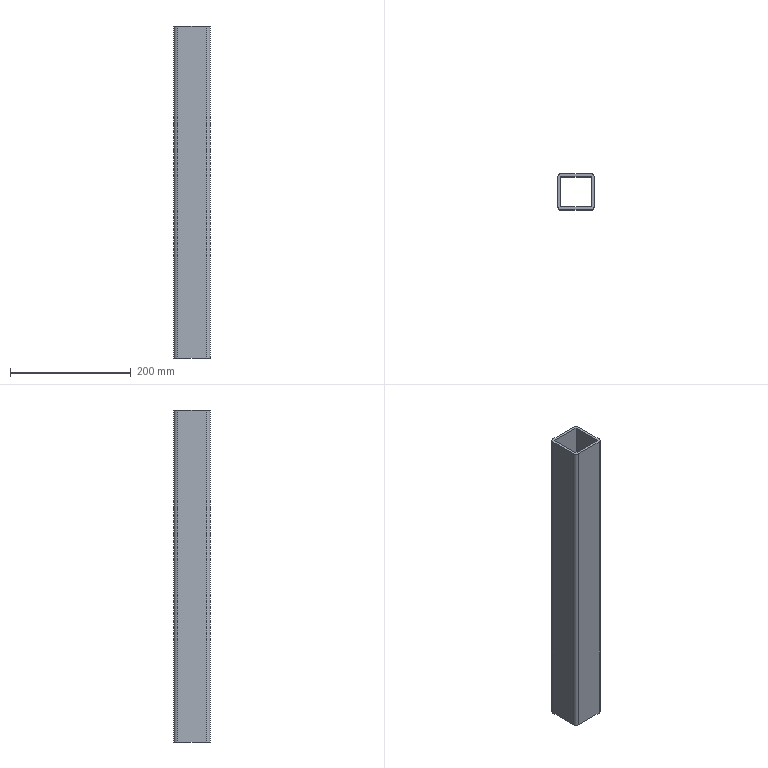Part | STEP file | Positioning_id154_x_t | 1 solid | 14 faces | box 60 x 60 x 550 mm | volume 588004 mm3 | plane 10 | cylinder 4 | commonest cylinder face diameters 12 x4
STEP:
#1=CARTESIAN_POINT('',(0.,0.,0.));
#2=DIRECTION('',(0.,0.,1.));
#3=DIRECTION('',(1.,0.,0.));
#4=AXIS2_PLACEMENT_3D('',#1,#2,#3);
#5=CARTESIAN_POINT('',(-1086.002,-25.,-77.534));
#6=VERTEX_POINT('',#5);
#7=CARTESIAN_POINT('',(-1086.002,25.,-77.534));
#8=VERTEX_POINT('',#7);
#9=CARTESIAN_POINT('',(-1086.002,-25.,-77.534));
#10=DIRECTION('',(0.,1.,0.));
#11=VECTOR('',#10,1.);
#12=LINE('',#9,#11);
#13=CARTESIAN_POINT('',(-1037.002,590.,-77.534));
#14=DIRECTION('',(0.,0.,1.));
#15=DIRECTION('',(-1.,0.,0.));
#16=AXIS2_PLACEMENT_3D('',#13,#14,#15);
#17=PLANE('',#16);
#18=CARTESIAN_POINT('',(49.,615.));
#19=DIRECTION('',(0.,-1.));
#20=VECTOR('',#19,1.);
#21=LINE('',#18,#20);
#22=(GEOMETRIC_REPRESENTATION_CONTEXT(2)PARAMETRIC_REPRESENTATION_CONTEXT()REPRESENTATION_CONTEXT('',''));
#23=DEFINITIONAL_REPRESENTATION('',(#21),#22);
#24=PCURVE('',#17,#23);
#25=CARTESIAN_POINT('',(-1086.002,-25.,197.466));
#26=DIRECTION('',(-1.,0.,0.));
#27=DIRECTION('',(0.,1.,0.));
#28=AXIS2_PLACEMENT_3D('',#25,#26,#27);
#29=PLANE('',#28);
#30=CARTESIAN_POINT('',(0.,275.));
#31=DIRECTION('',(1.,0.));
#32=VECTOR('',#31,1.);
#33=LINE('',#30,#32);
#34=(GEOMETRIC_REPRESENTATION_CONTEXT(2)PARAMETRIC_REPRESENTATION_CONTEXT()REPRESENTATION_CONTEXT('',''));
#35=DEFINITIONAL_REPRESENTATION('',(#33),#34);
#36=PCURVE('',#29,#35);
#37=SURFACE_CURVE('',#12,(#24,#36),.PCURVE_S1.);
#38=EDGE_CURVE('',#6,#8,#37,.T.);
#39=ORIENTED_EDGE('',*,*,#38,.F.);
#40=CARTESIAN_POINT('',(-1036.002,-25.,-77.534));
#41=VERTEX_POINT('',#40);
#42=CARTESIAN_POINT('',(-1036.002,-25.,-77.534));
#43=DIRECTION('',(-1.,0.,0.));
#44=VECTOR('',#43,1.);
#45=LINE('',#42,#44);
#46=CARTESIAN_POINT('',(-1.,615.));
#47=DIRECTION('',(1.,0.));
#48=VECTOR('',#47,1.);
#49=LINE('',#46,#48);
#50=(GEOMETRIC_REPRESENTATION_CONTEXT(2)PARAMETRIC_REPRESENTATION_CONTEXT()REPRESENTATION_CONTEXT('',''));
#51=DEFINITIONAL_REPRESENTATION('',(#49),#50);
#52=PCURVE('',#17,#51);
#53=CARTESIAN_POINT('',(-1061.002,-25.,197.466));
#54=DIRECTION('',(0.,-1.,0.));
#55=DIRECTION('',(-1.,0.,0.));
#56=AXIS2_PLACEMENT_3D('',#53,#54,#55);
#57=PLANE('',#56);
#58=CARTESIAN_POINT('',(-25.,275.));
#59=DIRECTION('',(1.,0.));
#60=VECTOR('',#59,1.);
#61=LINE('',#58,#60);
#62=(GEOMETRIC_REPRESENTATION_CONTEXT(2)PARAMETRIC_REPRESENTATION_CONTEXT()REPRESENTATION_CONTEXT('',''));
#63=DEFINITIONAL_REPRESENTATION('',(#61),#62);
#64=PCURVE('',#57,#63);
#65=SURFACE_CURVE('',#45,(#52,#64),.PCURVE_S1.);
#66=EDGE_CURVE('',#41,#6,#65,.T.);
#67=ORIENTED_EDGE('',*,*,#66,.F.);
#68=CARTESIAN_POINT('',(-1036.002,25.,-77.534));
#69=VERTEX_POINT('',#68);
#70=CARTESIAN_POINT('',(-1036.002,25.,-77.534));
#71=DIRECTION('',(0.,-1.,0.));
#72=VECTOR('',#71,1.);
#73=LINE('',#70,#72);
#74=CARTESIAN_POINT('',(-1.,565.));
#75=DIRECTION('',(0.,1.));
#76=VECTOR('',#75,1.);
#77=LINE('',#74,#76);
#78=(GEOMETRIC_REPRESENTATION_CONTEXT(2)PARAMETRIC_REPRESENTATION_CONTEXT()REPRESENTATION_CONTEXT('',''));
#79=DEFINITIONAL_REPRESENTATION('',(#77),#78);
#80=PCURVE('',#17,#79);
#81=CARTESIAN_POINT('',(-1036.002,-25.,197.466));
#82=DIRECTION('',(1.,0.,0.));
#83=DIRECTION('',(0.,-1.,0.));
#84=AXIS2_PLACEMENT_3D('',#81,#82,#83);
#85=PLANE('',#84);
#86=CARTESIAN_POINT('',(-50.,275.));
#87=DIRECTION('',(1.,0.));
#88=VECTOR('',#87,1.);
#89=LINE('',#86,#88);
#90=(GEOMETRIC_REPRESENTATION_CONTEXT(2)PARAMETRIC_REPRESENTATION_CONTEXT()REPRESENTATION_CONTEXT('',''));
#91=DEFINITIONAL_REPRESENTATION('',(#89),#90);
#92=PCURVE('',#85,#91);
#93=SURFACE_CURVE('',#73,(#80,#92),.PCURVE_S1.);
#94=EDGE_CURVE('',#69,#41,#93,.T.);
#95=ORIENTED_EDGE('',*,*,#94,.F.);
#96=CARTESIAN_POINT('',(-1086.002,25.,-77.534));
#97=DIRECTION('',(1.,0.,0.));
#98=VECTOR('',#97,1.);
#99=LINE('',#96,#98);
#100=CARTESIAN_POINT('',(49.,565.));
#101=DIRECTION('',(-1.,0.));
#102=VECTOR('',#101,1.);
#103=LINE('',#100,#102);
#104=(GEOMETRIC_REPRESENTATION_CONTEXT(2)PARAMETRIC_REPRESENTATION_CONTEXT()REPRESENTATION_CONTEXT('',''));
#105=DEFINITIONAL_REPRESENTATION('',(#103),#104);
#106=PCURVE('',#17,#105);
#107=CARTESIAN_POINT('',(-1061.002,25.,197.466));
#108=DIRECTION('',(0.,1.,0.));
#109=DIRECTION('',(1.,0.,0.));
#110=AXIS2_PLACEMENT_3D('',#107,#108,#109);
#111=PLANE('',#110);
#112=CARTESIAN_POINT('',(-25.,275.));
#113=DIRECTION('',(1.,0.));
#114=VECTOR('',#113,1.);
#115=LINE('',#112,#114);
#116=(GEOMETRIC_REPRESENTATION_CONTEXT(2)PARAMETRIC_REPRESENTATION_CONTEXT()REPRESENTATION_CONTEXT('',''));
#117=DEFINITIONAL_REPRESENTATION('',(#115),#116);
#118=PCURVE('',#111,#117);
#119=SURFACE_CURVE('',#99,(#106,#118),.PCURVE_S1.);
#120=EDGE_CURVE('',#8,#69,#119,.T.);
#121=ORIENTED_EDGE('',*,*,#120,.F.);
#122=EDGE_LOOP('',(#39,#67,#95,#121));
#123=FACE_BOUND('',#122,.T.);
#124=CARTESIAN_POINT('',(-1037.002,30.,-77.534));
#125=VERTEX_POINT('',#124);
#126=CARTESIAN_POINT('',(-1031.002,24.,-77.534));
#127=VERTEX_POINT('',#126);
#128=CARTESIAN_POINT('',(-1037.002,24.,-77.534));
#129=DIRECTION('',(0.,0.,-1.));
#130=DIRECTION('',(0.,1.,0.));
#131=AXIS2_PLACEMENT_3D('',#128,#129,#130);
#132=CIRCLE('',#131,6.);
#133=CARTESIAN_POINT('',(0.,560.));
#134=CARTESIAN_POINT('',(-10.392,560.));
#135=CARTESIAN_POINT('',(-5.196,569.));
#136=CARTESIAN_POINT('',(0.,578.));
#137=CARTESIAN_POINT('',(5.196,569.));
#138=CARTESIAN_POINT('',(10.392,560.));
#139=CARTESIAN_POINT('',(0.,560.));
#140=(BOUNDED_CURVE()B_SPLINE_CURVE(2,(#133,#134,#135,#136,#137,#138,#139),.UNSPECIFIED.,.T.,.F.)B_SPLINE_CURVE_WITH_KNOTS((1,2,2,2,2,1),(-2.094,0.,2.094,4.189,6.283,8.378),.UNSPECIFIED.)CURVE()GEOMETRIC_REPRESENTATION_ITEM()RATIONAL_B_SPLINE_CURVE((1.,0.5,1.,0.5,1.,0.5,1.))REPRESENTATION_ITEM(''));
#141=(GEOMETRIC_REPRESENTATION_CONTEXT(2)PARAMETRIC_REPRESENTATION_CONTEXT()REPRESENTATION_CONTEXT('',''));
#142=DEFINITIONAL_REPRESENTATION('',(#140),#141);
#143=PCURVE('',#17,#142);
#144=CARTESIAN_POINT('',(-1037.002,24.,197.466));
#145=DIRECTION('',(0.,0.,-1.));
#146=DIRECTION('',(-1.,0.,0.));
#147=AXIS2_PLACEMENT_3D('',#144,#145,#146);
#148=CYLINDRICAL_SURFACE('',#147,6.);
#149=CARTESIAN_POINT('',(1.571,275.));
#150=DIRECTION('',(1.,0.));
#151=VECTOR('',#150,1.);
#152=LINE('',#149,#151);
#153=(GEOMETRIC_REPRESENTATION_CONTEXT(2)PARAMETRIC_REPRESENTATION_CONTEXT()REPRESENTATION_CONTEXT('',''));
#154=DEFINITIONAL_REPRESENTATION('',(#152),#153);
#155=PCURVE('',#148,#154);
#156=SURFACE_CURVE('',#132,(#143,#155),.PCURVE_S1.);
#157=EDGE_CURVE('',#125,#127,#156,.T.);
#158=ORIENTED_EDGE('',*,*,#157,.T.);
#159=CARTESIAN_POINT('',(-1031.002,-24.,-77.534));
#160=VERTEX_POINT('',#159);
#161=CARTESIAN_POINT('',(-1031.002,24.,-77.534));
#162=DIRECTION('',(0.,-1.,0.));
#163=VECTOR('',#162,1.);
#164=LINE('',#161,#163);
#165=CARTESIAN_POINT('',(-6.,566.));
#166=DIRECTION('',(0.,1.));
#167=VECTOR('',#166,1.);
#168=LINE('',#165,#167);
#169=(GEOMETRIC_REPRESENTATION_CONTEXT(2)PARAMETRIC_REPRESENTATION_CONTEXT()REPRESENTATION_CONTEXT('',''));
#170=DEFINITIONAL_REPRESENTATION('',(#168),#169);
#171=PCURVE('',#17,#170);
#172=CARTESIAN_POINT('',(-1031.002,-30.,197.466));
#173=DIRECTION('',(1.,0.,0.));
#174=DIRECTION('',(0.,-1.,0.));
#175=AXIS2_PLACEMENT_3D('',#172,#173,#174);
#176=PLANE('',#175);
#177=CARTESIAN_POINT('',(-54.,275.));
#178=DIRECTION('',(1.,0.));
#179=VECTOR('',#178,1.);
#180=LINE('',#177,#179);
#181=(GEOMETRIC_REPRESENTATION_CONTEXT(2)PARAMETRIC_REPRESENTATION_CONTEXT()REPRESENTATION_CONTEXT('',''));
#182=DEFINITIONAL_REPRESENTATION('',(#180),#181);
#183=PCURVE('',#176,#182);
#184=SURFACE_CURVE('',#164,(#171,#183),.PCURVE_S1.);
#185=EDGE_CURVE('',#127,#160,#184,.T.);
#186=ORIENTED_EDGE('',*,*,#185,.T.);
#187=CARTESIAN_POINT('',(-1037.002,-30.,-77.534));
#188=VERTEX_POINT('',#187);
#189=CARTESIAN_POINT('',(-1037.002,-24.,-77.534));
#190=DIRECTION('',(0.,0.,-1.));
#191=DIRECTION('',(1.,0.,0.));
#192=AXIS2_PLACEMENT_3D('',#189,#190,#191);
#193=CIRCLE('',#192,6.);
#194=CARTESIAN_POINT('',(-6.,614.));
#195=CARTESIAN_POINT('',(-6.,624.392));
#196=CARTESIAN_POINT('',(3.,619.196));
#197=CARTESIAN_POINT('',(12.,614.));
#198=CARTESIAN_POINT('',(3.,608.804));
#199=CARTESIAN_POINT('',(-6.,603.608));
#200=CARTESIAN_POINT('',(-6.,614.));
#201=(BOUNDED_CURVE()B_SPLINE_CURVE(2,(#194,#195,#196,#197,#198,#199,#200),.UNSPECIFIED.,.T.,.F.)B_SPLINE_CURVE_WITH_KNOTS((1,2,2,2,2,1),(-2.094,0.,2.094,4.189,6.283,8.378),.UNSPECIFIED.)CURVE()GEOMETRIC_REPRESENTATION_ITEM()RATIONAL_B_SPLINE_CURVE((1.,0.5,1.,0.5,1.,0.5,1.))REPRESENTATION_ITEM(''));
#202=(GEOMETRIC_REPRESENTATION_CONTEXT(2)PARAMETRIC_REPRESENTATION_CONTEXT()REPRESENTATION_CONTEXT('',''));
#203=DEFINITIONAL_REPRESENTATION('',(#201),#202);
#204=PCURVE('',#17,#203);
#205=CARTESIAN_POINT('',(-1037.002,-24.,197.466));
#206=DIRECTION('',(0.,0.,1.));
#207=DIRECTION('',(1.,0.,0.));
#208=AXIS2_PLACEMENT_3D('',#205,#206,#207);
#209=CYLINDRICAL_SURFACE('',#208,6.);
#210=CARTESIAN_POINT('',(6.283,-275.));
#211=DIRECTION('',(-1.,0.));
#212=VECTOR('',#211,1.);
#213=LINE('',#210,#212);
#214=(GEOMETRIC_REPRESENTATION_CONTEXT(2)PARAMETRIC_REPRESENTATION_CONTEXT()REPRESENTATION_CONTEXT('',''));
#215=DEFINITIONAL_REPRESENTATION('',(#213),#214);
#216=PCURVE('',#209,#215);
#217=SURFACE_CURVE('',#193,(#204,#216),.PCURVE_S1.);
#218=EDGE_CURVE('',#160,#188,#217,.T.);
#219=ORIENTED_EDGE('',*,*,#218,.T.);
#220=CARTESIAN_POINT('',(-1085.002,-30.,-77.534));
#221=VERTEX_POINT('',#220);
#222=CARTESIAN_POINT('',(-1037.002,-30.,-77.534));
#223=DIRECTION('',(-1.,0.,0.));
#224=VECTOR('',#223,1.);
#225=LINE('',#222,#224);
#226=CARTESIAN_POINT('',(0.,620.));
#227=DIRECTION('',(1.,0.));
#228=VECTOR('',#227,1.);
#229=LINE('',#226,#228);
#230=(GEOMETRIC_REPRESENTATION_CONTEXT(2)PARAMETRIC_REPRESENTATION_CONTEXT()REPRESENTATION_CONTEXT('',''));
#231=DEFINITIONAL_REPRESENTATION('',(#229),#230);
#232=PCURVE('',#17,#231);
#233=CARTESIAN_POINT('',(-1061.002,-30.,197.466));
#234=DIRECTION('',(0.,-1.,0.));
#235=DIRECTION('',(-1.,0.,0.));
#236=AXIS2_PLACEMENT_3D('',#233,#234,#235);
#237=PLANE('',#236);
#238=CARTESIAN_POINT('',(-24.,275.));
#239=DIRECTION('',(1.,0.));
#240=VECTOR('',#239,1.);
#241=LINE('',#238,#240);
#242=(GEOMETRIC_REPRESENTATION_CONTEXT(2)PARAMETRIC_REPRESENTATION_CONTEXT()REPRESENTATION_CONTEXT('',''));
#243=DEFINITIONAL_REPRESENTATION('',(#241),#242);
#244=PCURVE('',#237,#243);
#245=SURFACE_CURVE('',#225,(#232,#244),.PCURVE_S1.);
#246=EDGE_CURVE('',#188,#221,#245,.T.);
#247=ORIENTED_EDGE('',*,*,#246,.T.);
#248=CARTESIAN_POINT('',(-1091.002,-24.,-77.534));
#249=VERTEX_POINT('',#248);
#250=CARTESIAN_POINT('',(-1085.002,-24.,-77.534));
#251=DIRECTION('',(0.,0.,-1.));
#252=DIRECTION('',(0.,-1.,0.));
#253=AXIS2_PLACEMENT_3D('',#250,#251,#252);
#254=CIRCLE('',#253,6.);
#255=CARTESIAN_POINT('',(48.,620.));
#256=CARTESIAN_POINT('',(58.392,620.));
#257=CARTESIAN_POINT('',(53.196,611.));
#258=CARTESIAN_POINT('',(48.,602.));
#259=CARTESIAN_POINT('',(42.804,611.));
#260=CARTESIAN_POINT('',(37.608,620.));
#261=CARTESIAN_POINT('',(48.,620.));
#262=(BOUNDED_CURVE()B_SPLINE_CURVE(2,(#255,#256,#257,#258,#259,#260,#261),.UNSPECIFIED.,.T.,.F.)B_SPLINE_CURVE_WITH_KNOTS((1,2,2,2,2,1),(-2.094,0.,2.094,4.189,6.283,8.378),.UNSPECIFIED.)CURVE()GEOMETRIC_REPRESENTATION_ITEM()RATIONAL_B_SPLINE_CURVE((1.,0.5,1.,0.5,1.,0.5,1.))REPRESENTATION_ITEM(''));
#263=(GEOMETRIC_REPRESENTATION_CONTEXT(2)PARAMETRIC_REPRESENTATION_CONTEXT()REPRESENTATION_CONTEXT('',''));
#264=DEFINITIONAL_REPRESENTATION('',(#262),#263);
#265=PCURVE('',#17,#264);
#266=CARTESIAN_POINT('',(-1085.002,-24.,197.466));
#267=DIRECTION('',(0.,0.,-1.));
#268=DIRECTION('',(-1.,0.,0.));
#269=AXIS2_PLACEMENT_3D('',#266,#267,#268);
#270=CYLINDRICAL_SURFACE('',#269,6.);
#271=CARTESIAN_POINT('',(4.712,275.));
#272=DIRECTION('',(1.,0.));
#273=VECTOR('',#272,1.);
#274=LINE('',#271,#273);
#275=(GEOMETRIC_REPRESENTATION_CONTEXT(2)PARAMETRIC_REPRESENTATION_CONTEXT()REPRESENTATION_CONTEXT('',''));
#276=DEFINITIONAL_REPRESENTATION('',(#274),#275);
#277=PCURVE('',#270,#276);
#278=SURFACE_CURVE('',#254,(#265,#277),.PCURVE_S1.);
#279=EDGE_CURVE('',#221,#249,#278,.T.);
#280=ORIENTED_EDGE('',*,*,#279,.T.);
#281=CARTESIAN_POINT('',(-1091.002,24.,-77.534));
#282=VERTEX_POINT('',#281);
#283=CARTESIAN_POINT('',(-1091.002,-24.,-77.534));
#284=DIRECTION('',(0.,1.,0.));
#285=VECTOR('',#284,1.);
#286=LINE('',#283,#285);
#287=CARTESIAN_POINT('',(54.,614.));
#288=DIRECTION('',(0.,-1.));
#289=VECTOR('',#288,1.);
#290=LINE('',#287,#289);
#291=(GEOMETRIC_REPRESENTATION_CONTEXT(2)PARAMETRIC_REPRESENTATION_CONTEXT()REPRESENTATION_CONTEXT('',''));
#292=DEFINITIONAL_REPRESENTATION('',(#290),#291);
#293=PCURVE('',#17,#292);
#294=CARTESIAN_POINT('',(-1091.002,-30.,197.466));
#295=DIRECTION('',(-1.,0.,0.));
#296=DIRECTION('',(0.,1.,0.));
#297=AXIS2_PLACEMENT_3D('',#294,#295,#296);
#298=PLANE('',#297);
#299=CARTESIAN_POINT('',(6.,275.));
#300=DIRECTION('',(1.,0.));
#301=VECTOR('',#300,1.);
#302=LINE('',#299,#301);
#303=(GEOMETRIC_REPRESENTATION_CONTEXT(2)PARAMETRIC_REPRESENTATION_CONTEXT()REPRESENTATION_CONTEXT('',''));
#304=DEFINITIONAL_REPRESENTATION('',(#302),#303);
#305=PCURVE('',#298,#304);
#306=SURFACE_CURVE('',#286,(#293,#305),.PCURVE_S1.);
#307=EDGE_CURVE('',#249,#282,#306,.T.);
#308=ORIENTED_EDGE('',*,*,#307,.T.);
#309=CARTESIAN_POINT('',(-1085.002,30.,-77.534));
#310=VERTEX_POINT('',#309);
#311=CARTESIAN_POINT('',(-1085.002,24.,-77.534));
#312=DIRECTION('',(0.,0.,-1.));
#313=DIRECTION('',(-1.,0.,0.));
#314=AXIS2_PLACEMENT_3D('',#311,#312,#313);
#315=CIRCLE('',#314,6.);
#316=CARTESIAN_POINT('',(54.,566.));
#317=CARTESIAN_POINT('',(54.,555.608));
#318=CARTESIAN_POINT('',(45.,560.804));
#319=CARTESIAN_POINT('',(36.,566.));
#320=CARTESIAN_POINT('',(45.,571.196));
#321=CARTESIAN_POINT('',(54.,576.392));
#322=CARTESIAN_POINT('',(54.,566.));
#323=(BOUNDED_CURVE()B_SPLINE_CURVE(2,(#316,#317,#318,#319,#320,#321,#322),.UNSPECIFIED.,.T.,.F.)B_SPLINE_CURVE_WITH_KNOTS((1,2,2,2,2,1),(-2.094,0.,2.094,4.189,6.283,8.378),.UNSPECIFIED.)CURVE()GEOMETRIC_REPRESENTATION_ITEM()RATIONAL_B_SPLINE_CURVE((1.,0.5,1.,0.5,1.,0.5,1.))REPRESENTATION_ITEM(''));
#324=(GEOMETRIC_REPRESENTATION_CONTEXT(2)PARAMETRIC_REPRESENTATION_CONTEXT()REPRESENTATION_CONTEXT('',''));
#325=DEFINITIONAL_REPRESENTATION('',(#323),#324);
#326=PCURVE('',#17,#325);
#327=CARTESIAN_POINT('',(-1085.002,24.,197.466));
#328=DIRECTION('',(0.,0.,1.));
#329=DIRECTION('',(1.,0.,0.));
#330=AXIS2_PLACEMENT_3D('',#327,#328,#329);
#331=CYLINDRICAL_SURFACE('',#330,6.);
#332=CARTESIAN_POINT('',(3.142,-275.));
#333=DIRECTION('',(-1.,0.));
#334=VECTOR('',#333,1.);
#335=LINE('',#332,#334);
#336=(GEOMETRIC_REPRESENTATION_CONTEXT(2)PARAMETRIC_REPRESENTATION_CONTEXT()REPRESENTATION_CONTEXT('',''));
#337=DEFINITIONAL_REPRESENTATION('',(#335),#336);
#338=PCURVE('',#331,#337);
#339=SURFACE_CURVE('',#315,(#326,#338),.PCURVE_S1.);
#340=EDGE_CURVE('',#282,#310,#339,.T.);
#341=ORIENTED_EDGE('',*,*,#340,.T.);
#342=CARTESIAN_POINT('',(-1085.002,30.,-77.534));
#343=DIRECTION('',(1.,0.,0.));
#344=VECTOR('',#343,1.);
#345=LINE('',#342,#344);
#346=CARTESIAN_POINT('',(48.,560.));
#347=DIRECTION('',(-1.,0.));
#348=VECTOR('',#347,1.);
#349=LINE('',#346,#348);
#350=(GEOMETRIC_REPRESENTATION_CONTEXT(2)PARAMETRIC_REPRESENTATION_CONTEXT()REPRESENTATION_CONTEXT('',''));
#351=DEFINITIONAL_REPRESENTATION('',(#349),#350);
#352=PCURVE('',#17,#351);
#353=CARTESIAN_POINT('',(-1061.002,30.,197.466));
#354=DIRECTION('',(0.,1.,0.));
#355=DIRECTION('',(1.,0.,0.));
#356=AXIS2_PLACEMENT_3D('',#353,#354,#355);
#357=PLANE('',#356);
#358=CARTESIAN_POINT('',(-24.,275.));
#359=DIRECTION('',(1.,0.));
#360=VECTOR('',#359,1.);
#361=LINE('',#358,#360);
#362=(GEOMETRIC_REPRESENTATION_CONTEXT(2)PARAMETRIC_REPRESENTATION_CONTEXT()REPRESENTATION_CONTEXT('',''));
#363=DEFINITIONAL_REPRESENTATION('',(#361),#362);
#364=PCURVE('',#357,#363);
#365=SURFACE_CURVE('',#345,(#352,#364),.PCURVE_S1.);
#366=EDGE_CURVE('',#310,#125,#365,.T.);
#367=ORIENTED_EDGE('',*,*,#366,.T.);
#368=EDGE_LOOP('',(#158,#186,#219,#247,#280,#308,#341,#367));
#369=FACE_BOUND('',#368,.T.);
#370=ADVANCED_FACE('',(#123,#369),#17,.F.);
#371=CARTESIAN_POINT('',(-1036.002,-25.,472.466));
#372=VERTEX_POINT('',#371);
#373=CARTESIAN_POINT('',(-1036.002,25.,472.466));
#374=VERTEX_POINT('',#373);
#375=CARTESIAN_POINT('',(-1036.002,-25.,472.466));
#376=DIRECTION('',(0.,1.,0.));
#377=VECTOR('',#376,1.);
#378=LINE('',#375,#377);
#379=CARTESIAN_POINT('',(-1037.002,-590.,472.466));
#380=DIRECTION('',(0.,0.,-1.));
#381=DIRECTION('',(1.,0.,0.));
#382=AXIS2_PLACEMENT_3D('',#379,#380,#381);
#383=PLANE('',#382);
#384=CARTESIAN_POINT('',(1.,-565.));
#385=DIRECTION('',(0.,-1.));
#386=VECTOR('',#385,1.);
#387=LINE('',#384,#386);
#388=(GEOMETRIC_REPRESENTATION_CONTEXT(2)PARAMETRIC_REPRESENTATION_CONTEXT()REPRESENTATION_CONTEXT('',''));
#389=DEFINITIONAL_REPRESENTATION('',(#387),#388);
#390=PCURVE('',#383,#389);
#391=CARTESIAN_POINT('',(0.,-275.));
#392=DIRECTION('',(-1.,0.));
#393=VECTOR('',#392,1.);
#394=LINE('',#391,#393);
#395=(GEOMETRIC_REPRESENTATION_CONTEXT(2)PARAMETRIC_REPRESENTATION_CONTEXT()REPRESENTATION_CONTEXT('',''));
#396=DEFINITIONAL_REPRESENTATION('',(#394),#395);
#397=PCURVE('',#85,#396);
#398=SURFACE_CURVE('',#378,(#390,#397),.PCURVE_S1.);
#399=EDGE_CURVE('',#372,#374,#398,.T.);
#400=ORIENTED_EDGE('',*,*,#399,.F.);
#401=CARTESIAN_POINT('',(-1086.002,-25.,472.466));
#402=VERTEX_POINT('',#401);
#403=CARTESIAN_POINT('',(-1086.002,-25.,472.466));
#404=DIRECTION('',(1.,0.,0.));
#405=VECTOR('',#404,1.);
#406=LINE('',#403,#405);
#407=CARTESIAN_POINT('',(-49.,-565.));
#408=DIRECTION('',(1.,0.));
#409=VECTOR('',#408,1.);
#410=LINE('',#407,#409);
#411=(GEOMETRIC_REPRESENTATION_CONTEXT(2)PARAMETRIC_REPRESENTATION_CONTEXT()REPRESENTATION_CONTEXT('',''));
#412=DEFINITIONAL_REPRESENTATION('',(#410),#411);
#413=PCURVE('',#383,#412);
#414=CARTESIAN_POINT('',(25.,-275.));
#415=DIRECTION('',(-1.,0.));
#416=VECTOR('',#415,1.);
#417=LINE('',#414,#416);
#418=(GEOMETRIC_REPRESENTATION_CONTEXT(2)PARAMETRIC_REPRESENTATION_CONTEXT()REPRESENTATION_CONTEXT('',''));
#419=DEFINITIONAL_REPRESENTATION('',(#417),#418);
#420=PCURVE('',#57,#419);
#421=SURFACE_CURVE('',#406,(#413,#420),.PCURVE_S1.);
#422=EDGE_CURVE('',#402,#372,#421,.T.);
#423=ORIENTED_EDGE('',*,*,#422,.F.);
#424=CARTESIAN_POINT('',(-1086.002,25.,472.466));
#425=VERTEX_POINT('',#424);
#426=CARTESIAN_POINT('',(-1086.002,25.,472.466));
#427=DIRECTION('',(0.,-1.,0.));
#428=VECTOR('',#427,1.);
#429=LINE('',#426,#428);
#430=CARTESIAN_POINT('',(-49.,-615.));
#431=DIRECTION('',(0.,1.));
#432=VECTOR('',#431,1.);
#433=LINE('',#430,#432);
#434=(GEOMETRIC_REPRESENTATION_CONTEXT(2)PARAMETRIC_REPRESENTATION_CONTEXT()REPRESENTATION_CONTEXT('',''));
#435=DEFINITIONAL_REPRESENTATION('',(#433),#434);
#436=PCURVE('',#383,#435);
#437=CARTESIAN_POINT('',(50.,-275.));
#438=DIRECTION('',(-1.,0.));
#439=VECTOR('',#438,1.);
#440=LINE('',#437,#439);
#441=(GEOMETRIC_REPRESENTATION_CONTEXT(2)PARAMETRIC_REPRESENTATION_CONTEXT()REPRESENTATION_CONTEXT('',''));
#442=DEFINITIONAL_REPRESENTATION('',(#440),#441);
#443=PCURVE('',#29,#442);
#444=SURFACE_CURVE('',#429,(#436,#443),.PCURVE_S1.);
#445=EDGE_CURVE('',#425,#402,#444,.T.);
#446=ORIENTED_EDGE('',*,*,#445,.F.);
#447=CARTESIAN_POINT('',(-1036.002,25.,472.466));
#448=DIRECTION('',(-1.,0.,0.));
#449=VECTOR('',#448,1.);
#450=LINE('',#447,#449);
#451=CARTESIAN_POINT('',(1.,-615.));
#452=DIRECTION('',(-1.,0.));
#453=VECTOR('',#452,1.);
#454=LINE('',#451,#453);
#455=(GEOMETRIC_REPRESENTATION_CONTEXT(2)PARAMETRIC_REPRESENTATION_CONTEXT()REPRESENTATION_CONTEXT('',''));
#456=DEFINITIONAL_REPRESENTATION('',(#454),#455);
#457=PCURVE('',#383,#456);
#458=CARTESIAN_POINT('',(25.,-275.));
#459=DIRECTION('',(-1.,0.));
#460=VECTOR('',#459,1.);
#461=LINE('',#458,#460);
#462=(GEOMETRIC_REPRESENTATION_CONTEXT(2)PARAMETRIC_REPRESENTATION_CONTEXT()REPRESENTATION_CONTEXT('',''));
#463=DEFINITIONAL_REPRESENTATION('',(#461),#462);
#464=PCURVE('',#111,#463);
#465=SURFACE_CURVE('',#450,(#457,#464),.PCURVE_S1.);
#466=EDGE_CURVE('',#374,#425,#465,.T.);
#467=ORIENTED_EDGE('',*,*,#466,.F.);
#468=EDGE_LOOP('',(#400,#423,#446,#467));
#469=FACE_BOUND('',#468,.T.);
#470=CARTESIAN_POINT('',(-1031.002,24.,472.466));
#471=VERTEX_POINT('',#470);
#472=CARTESIAN_POINT('',(-1037.002,30.,472.466));
#473=VERTEX_POINT('',#472);
#474=CARTESIAN_POINT('',(-1037.002,24.,472.466));
#475=DIRECTION('',(0.,0.,1.));
#476=DIRECTION('',(1.,0.,0.));
#477=AXIS2_PLACEMENT_3D('',#474,#475,#476);
#478=CIRCLE('',#477,6.);
#479=CARTESIAN_POINT('',(6.,-614.));
#480=CARTESIAN_POINT('',(6.,-624.392));
#481=CARTESIAN_POINT('',(-3.,-619.196));
#482=CARTESIAN_POINT('',(-12.,-614.));
#483=CARTESIAN_POINT('',(-3.,-608.804));
#484=CARTESIAN_POINT('',(6.,-603.608));
#485=CARTESIAN_POINT('',(6.,-614.));
#486=(BOUNDED_CURVE()B_SPLINE_CURVE(2,(#479,#480,#481,#482,#483,#484,#485),.UNSPECIFIED.,.T.,.F.)B_SPLINE_CURVE_WITH_KNOTS((1,2,2,2,2,1),(-2.094,0.,2.094,4.189,6.283,8.378),.UNSPECIFIED.)CURVE()GEOMETRIC_REPRESENTATION_ITEM()RATIONAL_B_SPLINE_CURVE((1.,0.5,1.,0.5,1.,0.5,1.))REPRESENTATION_ITEM(''));
#487=(GEOMETRIC_REPRESENTATION_CONTEXT(2)PARAMETRIC_REPRESENTATION_CONTEXT()REPRESENTATION_CONTEXT('',''));
#488=DEFINITIONAL_REPRESENTATION('',(#486),#487);
#489=PCURVE('',#383,#488);
#490=CARTESIAN_POINT('',(3.142,-275.));
#491=DIRECTION('',(-1.,0.));
#492=VECTOR('',#491,1.);
#493=LINE('',#490,#492);
#494=(GEOMETRIC_REPRESENTATION_CONTEXT(2)PARAMETRIC_REPRESENTATION_CONTEXT()REPRESENTATION_CONTEXT('',''));
#495=DEFINITIONAL_REPRESENTATION('',(#493),#494);
#496=PCURVE('',#148,#495);
#497=SURFACE_CURVE('',#478,(#489,#496),.PCURVE_S1.);
#498=EDGE_CURVE('',#471,#473,#497,.T.);
#499=ORIENTED_EDGE('',*,*,#498,.T.);
#500=CARTESIAN_POINT('',(-1085.002,30.,472.466));
#501=VERTEX_POINT('',#500);
#502=CARTESIAN_POINT('',(-1085.002,30.,472.466));
#503=DIRECTION('',(1.,0.,0.));
#504=VECTOR('',#503,1.);
#505=LINE('',#502,#504);
#506=CARTESIAN_POINT('',(-48.,-620.));
#507=DIRECTION('',(1.,0.));
#508=VECTOR('',#507,1.);
#509=LINE('',#506,#508);
#510=(GEOMETRIC_REPRESENTATION_CONTEXT(2)PARAMETRIC_REPRESENTATION_CONTEXT()REPRESENTATION_CONTEXT('',''));
#511=DEFINITIONAL_REPRESENTATION('',(#509),#510);
#512=PCURVE('',#383,#511);
#513=CARTESIAN_POINT('',(-24.,-275.));
#514=DIRECTION('',(1.,0.));
#515=VECTOR('',#514,1.);
#516=LINE('',#513,#515);
#517=(GEOMETRIC_REPRESENTATION_CONTEXT(2)PARAMETRIC_REPRESENTATION_CONTEXT()REPRESENTATION_CONTEXT('',''));
#518=DEFINITIONAL_REPRESENTATION('',(#516),#517);
#519=PCURVE('',#357,#518);
#520=SURFACE_CURVE('',#505,(#512,#519),.PCURVE_S1.);
#521=EDGE_CURVE('',#501,#473,#520,.T.);
#522=ORIENTED_EDGE('',*,*,#521,.F.);
#523=CARTESIAN_POINT('',(-1091.002,24.,472.466));
#524=VERTEX_POINT('',#523);
#525=CARTESIAN_POINT('',(-1085.002,24.,472.466));
#526=DIRECTION('',(0.,0.,1.));
#527=DIRECTION('',(0.,1.,0.));
#528=AXIS2_PLACEMENT_3D('',#525,#526,#527);
#529=CIRCLE('',#528,6.);
#530=CARTESIAN_POINT('',(-48.,-620.));
#531=CARTESIAN_POINT('',(-58.392,-620.));
#532=CARTESIAN_POINT('',(-53.196,-611.));
#533=CARTESIAN_POINT('',(-48.,-602.));
#534=CARTESIAN_POINT('',(-42.804,-611.));
#535=CARTESIAN_POINT('',(-37.608,-620.));
#536=CARTESIAN_POINT('',(-48.,-620.));
#537=(BOUNDED_CURVE()B_SPLINE_CURVE(2,(#530,#531,#532,#533,#534,#535,#536),.UNSPECIFIED.,.T.,.F.)B_SPLINE_CURVE_WITH_KNOTS((1,2,2,2,2,1),(-2.094,0.,2.094,4.189,6.283,8.378),.UNSPECIFIED.)CURVE()GEOMETRIC_REPRESENTATION_ITEM()RATIONAL_B_SPLINE_CURVE((1.,0.5,1.,0.5,1.,0.5,1.))REPRESENTATION_ITEM(''));
#538=(GEOMETRIC_REPRESENTATION_CONTEXT(2)PARAMETRIC_REPRESENTATION_CONTEXT()REPRESENTATION_CONTEXT('',''));
#539=DEFINITIONAL_REPRESENTATION('',(#537),#538);
#540=PCURVE('',#383,#539);
#541=CARTESIAN_POINT('',(1.571,275.));
#542=DIRECTION('',(1.,0.));
#543=VECTOR('',#542,1.);
#544=LINE('',#541,#543);
#545=(GEOMETRIC_REPRESENTATION_CONTEXT(2)PARAMETRIC_REPRESENTATION_CONTEXT()REPRESENTATION_CONTEXT('',''));
#546=DEFINITIONAL_REPRESENTATION('',(#544),#545);
#547=PCURVE('',#331,#546);
#548=SURFACE_CURVE('',#529,(#540,#547),.PCURVE_S1.);
#549=EDGE_CURVE('',#501,#524,#548,.T.);
#550=ORIENTED_EDGE('',*,*,#549,.T.);
#551=CARTESIAN_POINT('',(-1091.002,-24.,472.466));
#552=VERTEX_POINT('',#551);
#553=CARTESIAN_POINT('',(-1091.002,24.,472.466));
#554=DIRECTION('',(0.,-1.,0.));
#555=VECTOR('',#554,1.);
#556=LINE('',#553,#555);
#557=CARTESIAN_POINT('',(-54.,-614.));
#558=DIRECTION('',(0.,1.));
#559=VECTOR('',#558,1.);
#560=LINE('',#557,#559);
#561=(GEOMETRIC_REPRESENTATION_CONTEXT(2)PARAMETRIC_REPRESENTATION_CONTEXT()REPRESENTATION_CONTEXT('',''));
#562=DEFINITIONAL_REPRESENTATION('',(#560),#561);
#563=PCURVE('',#383,#562);
#564=CARTESIAN_POINT('',(54.,-275.));
#565=DIRECTION('',(-1.,0.));
#566=VECTOR('',#565,1.);
#567=LINE('',#564,#566);
#568=(GEOMETRIC_REPRESENTATION_CONTEXT(2)PARAMETRIC_REPRESENTATION_CONTEXT()REPRESENTATION_CONTEXT('',''));
#569=DEFINITIONAL_REPRESENTATION('',(#567),#568);
#570=PCURVE('',#298,#569);
#571=SURFACE_CURVE('',#556,(#563,#570),.PCURVE_S1.);
#572=EDGE_CURVE('',#524,#552,#571,.T.);
#573=ORIENTED_EDGE('',*,*,#572,.T.);
#574=CARTESIAN_POINT('',(-1085.002,-30.,472.466));
#575=VERTEX_POINT('',#574);
#576=CARTESIAN_POINT('',(-1085.002,-24.,472.466));
#577=DIRECTION('',(0.,0.,1.));
#578=DIRECTION('',(-1.,0.,0.));
#579=AXIS2_PLACEMENT_3D('',#576,#577,#578);
#580=CIRCLE('',#579,6.);
#581=CARTESIAN_POINT('',(-54.,-566.));
#582=CARTESIAN_POINT('',(-54.,-555.608));
#583=CARTESIAN_POINT('',(-45.,-560.804));
#584=CARTESIAN_POINT('',(-36.,-566.));
#585=CARTESIAN_POINT('',(-45.,-571.196));
#586=CARTESIAN_POINT('',(-54.,-576.392));
#587=CARTESIAN_POINT('',(-54.,-566.));
#588=(BOUNDED_CURVE()B_SPLINE_CURVE(2,(#581,#582,#583,#584,#585,#586,#587),.UNSPECIFIED.,.T.,.F.)B_SPLINE_CURVE_WITH_KNOTS((1,2,2,2,2,1),(-2.094,0.,2.094,4.189,6.283,8.378),.UNSPECIFIED.)CURVE()GEOMETRIC_REPRESENTATION_ITEM()RATIONAL_B_SPLINE_CURVE((1.,0.5,1.,0.5,1.,0.5,1.))REPRESENTATION_ITEM(''));
#589=(GEOMETRIC_REPRESENTATION_CONTEXT(2)PARAMETRIC_REPRESENTATION_CONTEXT()REPRESENTATION_CONTEXT('',''));
#590=DEFINITIONAL_REPRESENTATION('',(#588),#589);
#591=PCURVE('',#383,#590);
#592=CARTESIAN_POINT('',(6.283,-275.));
#593=DIRECTION('',(-1.,0.));
#594=VECTOR('',#593,1.);
#595=LINE('',#592,#594);
#596=(GEOMETRIC_REPRESENTATION_CONTEXT(2)PARAMETRIC_REPRESENTATION_CONTEXT()REPRESENTATION_CONTEXT('',''));
#597=DEFINITIONAL_REPRESENTATION('',(#595),#596);
#598=PCURVE('',#270,#597);
#599=SURFACE_CURVE('',#580,(#591,#598),.PCURVE_S1.);
#600=EDGE_CURVE('',#552,#575,#599,.T.);
#601=ORIENTED_EDGE('',*,*,#600,.T.);
#602=CARTESIAN_POINT('',(-1037.002,-30.,472.466));
#603=VERTEX_POINT('',#602);
#604=CARTESIAN_POINT('',(-1085.002,-30.,472.466));
#605=DIRECTION('',(1.,0.,0.));
#606=VECTOR('',#605,1.);
#607=LINE('',#604,#606);
#608=CARTESIAN_POINT('',(-48.,-560.));
#609=DIRECTION('',(1.,0.));
#610=VECTOR('',#609,1.);
#611=LINE('',#608,#610);
#612=(GEOMETRIC_REPRESENTATION_CONTEXT(2)PARAMETRIC_REPRESENTATION_CONTEXT()REPRESENTATION_CONTEXT('',''));
#613=DEFINITIONAL_REPRESENTATION('',(#611),#612);
#614=PCURVE('',#383,#613);
#615=CARTESIAN_POINT('',(24.,-275.));
#616=DIRECTION('',(-1.,0.));
#617=VECTOR('',#616,1.);
#618=LINE('',#615,#617);
#619=(GEOMETRIC_REPRESENTATION_CONTEXT(2)PARAMETRIC_REPRESENTATION_CONTEXT()REPRESENTATION_CONTEXT('',''));
#620=DEFINITIONAL_REPRESENTATION('',(#618),#619);
#621=PCURVE('',#237,#620);
#622=SURFACE_CURVE('',#607,(#614,#621),.PCURVE_S1.);
#623=EDGE_CURVE('',#575,#603,#622,.T.);
#624=ORIENTED_EDGE('',*,*,#623,.T.);
#625=CARTESIAN_POINT('',(-1031.002,-24.,472.466));
#626=VERTEX_POINT('',#625);
#627=CARTESIAN_POINT('',(-1037.002,-24.,472.466));
#628=DIRECTION('',(0.,0.,1.));
#629=DIRECTION('',(0.,-1.,0.));
#630=AXIS2_PLACEMENT_3D('',#627,#628,#629);
#631=CIRCLE('',#630,6.);
#632=CARTESIAN_POINT('',(0.,-560.));
#633=CARTESIAN_POINT('',(10.392,-560.));
#634=CARTESIAN_POINT('',(5.196,-569.));
#635=CARTESIAN_POINT('',(0.,-578.));
#636=CARTESIAN_POINT('',(-5.196,-569.));
#637=CARTESIAN_POINT('',(-10.392,-560.));
#638=CARTESIAN_POINT('',(0.,-560.));
#639=(BOUNDED_CURVE()B_SPLINE_CURVE(2,(#632,#633,#634,#635,#636,#637,#638),.UNSPECIFIED.,.T.,.F.)B_SPLINE_CURVE_WITH_KNOTS((1,2,2,2,2,1),(-2.094,0.,2.094,4.189,6.283,8.378),.UNSPECIFIED.)CURVE()GEOMETRIC_REPRESENTATION_ITEM()RATIONAL_B_SPLINE_CURVE((1.,0.5,1.,0.5,1.,0.5,1.))REPRESENTATION_ITEM(''));
#640=(GEOMETRIC_REPRESENTATION_CONTEXT(2)PARAMETRIC_REPRESENTATION_CONTEXT()REPRESENTATION_CONTEXT('',''));
#641=DEFINITIONAL_REPRESENTATION('',(#639),#640);
#642=PCURVE('',#383,#641);
#643=CARTESIAN_POINT('',(4.712,275.));
#644=DIRECTION('',(1.,0.));
#645=VECTOR('',#644,1.);
#646=LINE('',#643,#645);
#647=(GEOMETRIC_REPRESENTATION_CONTEXT(2)PARAMETRIC_REPRESENTATION_CONTEXT()REPRESENTATION_CONTEXT('',''));
#648=DEFINITIONAL_REPRESENTATION('',(#646),#647);
#649=PCURVE('',#209,#648);
#650=SURFACE_CURVE('',#631,(#642,#649),.PCURVE_S1.);
#651=EDGE_CURVE('',#603,#626,#650,.T.);
#652=ORIENTED_EDGE('',*,*,#651,.T.);
#653=CARTESIAN_POINT('',(-1031.002,-24.,472.466));
#654=DIRECTION('',(0.,1.,0.));
#655=VECTOR('',#654,1.);
#656=LINE('',#653,#655);
#657=CARTESIAN_POINT('',(6.,-566.));
#658=DIRECTION('',(0.,-1.));
#659=VECTOR('',#658,1.);
#660=LINE('',#657,#659);
#661=(GEOMETRIC_REPRESENTATION_CONTEXT(2)PARAMETRIC_REPRESENTATION_CONTEXT()REPRESENTATION_CONTEXT('',''));
#662=DEFINITIONAL_REPRESENTATION('',(#660),#661);
#663=PCURVE('',#383,#662);
#664=CARTESIAN_POINT('',(-6.,-275.));
#665=DIRECTION('',(-1.,0.));
#666=VECTOR('',#665,1.);
#667=LINE('',#664,#666);
#668=(GEOMETRIC_REPRESENTATION_CONTEXT(2)PARAMETRIC_REPRESENTATION_CONTEXT()REPRESENTATION_CONTEXT('',''));
#669=DEFINITIONAL_REPRESENTATION('',(#667),#668);
#670=PCURVE('',#176,#669);
#671=SURFACE_CURVE('',#656,(#663,#670),.PCURVE_S1.);
#672=EDGE_CURVE('',#626,#471,#671,.T.);
#673=ORIENTED_EDGE('',*,*,#672,.T.);
#674=EDGE_LOOP('',(#499,#522,#550,#573,#601,#624,#652,#673));
#675=FACE_BOUND('',#674,.T.);
#676=ADVANCED_FACE('',(#469,#675),#383,.F.);
#677=ORIENTED_EDGE('',*,*,#279,.F.);
#678=CARTESIAN_POINT('',(-1085.002,-30.,472.466));
#679=DIRECTION('',(0.,0.,-1.));
#680=VECTOR('',#679,1.);
#681=LINE('',#678,#680);
#682=CARTESIAN_POINT('',(4.712,-275.));
#683=DIRECTION('',(0.,1.));
#684=VECTOR('',#683,1.);
#685=LINE('',#682,#684);
#686=(GEOMETRIC_REPRESENTATION_CONTEXT(2)PARAMETRIC_REPRESENTATION_CONTEXT()REPRESENTATION_CONTEXT('',''));
#687=DEFINITIONAL_REPRESENTATION('',(#685),#686);
#688=PCURVE('',#270,#687);
#689=CARTESIAN_POINT('',(24.,-275.));
#690=DIRECTION('',(0.,1.));
#691=VECTOR('',#690,1.);
#692=LINE('',#689,#691);
#693=(GEOMETRIC_REPRESENTATION_CONTEXT(2)PARAMETRIC_REPRESENTATION_CONTEXT()REPRESENTATION_CONTEXT('',''));
#694=DEFINITIONAL_REPRESENTATION('',(#692),#693);
#695=PCURVE('',#237,#694);
#696=SURFACE_CURVE('',#681,(#688,#695),.PCURVE_S1.);
#697=EDGE_CURVE('',#575,#221,#696,.T.);
#698=ORIENTED_EDGE('',*,*,#697,.F.);
#699=ORIENTED_EDGE('',*,*,#600,.F.);
#700=CARTESIAN_POINT('',(-1091.002,-24.,-77.534));
#701=DIRECTION('',(0.,0.,1.));
#702=VECTOR('',#701,1.);
#703=LINE('',#700,#702);
#704=CARTESIAN_POINT('',(6.283,275.));
#705=DIRECTION('',(0.,-1.));
#706=VECTOR('',#705,1.);
#707=LINE('',#704,#706);
#708=(GEOMETRIC_REPRESENTATION_CONTEXT(2)PARAMETRIC_REPRESENTATION_CONTEXT()REPRESENTATION_CONTEXT('',''));
#709=DEFINITIONAL_REPRESENTATION('',(#707),#708);
#710=PCURVE('',#270,#709);
#711=CARTESIAN_POINT('',(6.,275.));
#712=DIRECTION('',(0.,-1.));
#713=VECTOR('',#712,1.);
#714=LINE('',#711,#713);
#715=(GEOMETRIC_REPRESENTATION_CONTEXT(2)PARAMETRIC_REPRESENTATION_CONTEXT()REPRESENTATION_CONTEXT('',''));
#716=DEFINITIONAL_REPRESENTATION('',(#714),#715);
#717=PCURVE('',#298,#716);
#718=SURFACE_CURVE('',#703,(#710,#717),.PCURVE_S1.);
#719=EDGE_CURVE('',#249,#552,#718,.T.);
#720=ORIENTED_EDGE('',*,*,#719,.F.);
#721=EDGE_LOOP('',(#677,#698,#699,#720));
#722=FACE_BOUND('',#721,.T.);
#723=ADVANCED_FACE('',(#722),#270,.T.);
#724=ORIENTED_EDGE('',*,*,#218,.F.);
#725=CARTESIAN_POINT('',(-1031.002,-24.,472.466));
#726=DIRECTION('',(0.,0.,-1.));
#727=VECTOR('',#726,1.);
#728=LINE('',#725,#727);
#729=CARTESIAN_POINT('',(6.283,275.));
#730=DIRECTION('',(0.,-1.));
#731=VECTOR('',#730,1.);
#732=LINE('',#729,#731);
#733=(GEOMETRIC_REPRESENTATION_CONTEXT(2)PARAMETRIC_REPRESENTATION_CONTEXT()REPRESENTATION_CONTEXT('',''));
#734=DEFINITIONAL_REPRESENTATION('',(#732),#733);
#735=PCURVE('',#209,#734);
#736=CARTESIAN_POINT('',(-6.,-275.));
#737=DIRECTION('',(0.,1.));
#738=VECTOR('',#737,1.);
#739=LINE('',#736,#738);
#740=(GEOMETRIC_REPRESENTATION_CONTEXT(2)PARAMETRIC_REPRESENTATION_CONTEXT()REPRESENTATION_CONTEXT('',''));
#741=DEFINITIONAL_REPRESENTATION('',(#739),#740);
#742=PCURVE('',#176,#741);
#743=SURFACE_CURVE('',#728,(#735,#742),.PCURVE_S1.);
#744=EDGE_CURVE('',#626,#160,#743,.T.);
#745=ORIENTED_EDGE('',*,*,#744,.F.);
#746=ORIENTED_EDGE('',*,*,#651,.F.);
#747=CARTESIAN_POINT('',(-1037.002,-30.,-77.534));
#748=DIRECTION('',(0.,0.,1.));
#749=VECTOR('',#748,1.);
#750=LINE('',#747,#749);
#751=CARTESIAN_POINT('',(4.712,-275.));
#752=DIRECTION('',(0.,1.));
#753=VECTOR('',#752,1.);
#754=LINE('',#751,#753);
#755=(GEOMETRIC_REPRESENTATION_CONTEXT(2)PARAMETRIC_REPRESENTATION_CONTEXT()REPRESENTATION_CONTEXT('',''));
#756=DEFINITIONAL_REPRESENTATION('',(#754),#755);
#757=PCURVE('',#209,#756);
#758=CARTESIAN_POINT('',(-24.,275.));
#759=DIRECTION('',(0.,-1.));
#760=VECTOR('',#759,1.);
#761=LINE('',#758,#760);
#762=(GEOMETRIC_REPRESENTATION_CONTEXT(2)PARAMETRIC_REPRESENTATION_CONTEXT()REPRESENTATION_CONTEXT('',''));
#763=DEFINITIONAL_REPRESENTATION('',(#761),#762);
#764=PCURVE('',#237,#763);
#765=SURFACE_CURVE('',#750,(#757,#764),.PCURVE_S1.);
#766=EDGE_CURVE('',#188,#603,#765,.T.);
#767=ORIENTED_EDGE('',*,*,#766,.F.);
#768=EDGE_LOOP('',(#724,#745,#746,#767));
#769=FACE_BOUND('',#768,.T.);
#770=ADVANCED_FACE('',(#769),#209,.T.);
#771=ORIENTED_EDGE('',*,*,#340,.F.);
#772=CARTESIAN_POINT('',(-1091.002,24.,472.466));
#773=DIRECTION('',(0.,0.,-1.));
#774=VECTOR('',#773,1.);
#775=LINE('',#772,#774);
#776=CARTESIAN_POINT('',(3.142,275.));
#777=DIRECTION('',(0.,-1.));
#778=VECTOR('',#777,1.);
#779=LINE('',#776,#778);
#780=(GEOMETRIC_REPRESENTATION_CONTEXT(2)PARAMETRIC_REPRESENTATION_CONTEXT()REPRESENTATION_CONTEXT('',''));
#781=DEFINITIONAL_REPRESENTATION('',(#779),#780);
#782=PCURVE('',#331,#781);
#783=CARTESIAN_POINT('',(54.,-275.));
#784=DIRECTION('',(0.,1.));
#785=VECTOR('',#784,1.);
#786=LINE('',#783,#785);
#787=(GEOMETRIC_REPRESENTATION_CONTEXT(2)PARAMETRIC_REPRESENTATION_CONTEXT()REPRESENTATION_CONTEXT('',''));
#788=DEFINITIONAL_REPRESENTATION('',(#786),#787);
#789=PCURVE('',#298,#788);
#790=SURFACE_CURVE('',#775,(#782,#789),.PCURVE_S1.);
#791=EDGE_CURVE('',#524,#282,#790,.T.);
#792=ORIENTED_EDGE('',*,*,#791,.F.);
#793=ORIENTED_EDGE('',*,*,#549,.F.);
#794=CARTESIAN_POINT('',(-1085.002,30.,-77.534));
#795=DIRECTION('',(0.,0.,1.));
#796=VECTOR('',#795,1.);
#797=LINE('',#794,#796);
#798=CARTESIAN_POINT('',(1.571,-275.));
#799=DIRECTION('',(0.,1.));
#800=VECTOR('',#799,1.);
#801=LINE('',#798,#800);
#802=(GEOMETRIC_REPRESENTATION_CONTEXT(2)PARAMETRIC_REPRESENTATION_CONTEXT()REPRESENTATION_CONTEXT('',''));
#803=DEFINITIONAL_REPRESENTATION('',(#801),#802);
#804=PCURVE('',#331,#803);
#805=CARTESIAN_POINT('',(-24.,275.));
#806=DIRECTION('',(0.,-1.));
#807=VECTOR('',#806,1.);
#808=LINE('',#805,#807);
#809=(GEOMETRIC_REPRESENTATION_CONTEXT(2)PARAMETRIC_REPRESENTATION_CONTEXT()REPRESENTATION_CONTEXT('',''));
#810=DEFINITIONAL_REPRESENTATION('',(#808),#809);
#811=PCURVE('',#357,#810);
#812=SURFACE_CURVE('',#797,(#804,#811),.PCURVE_S1.);
#813=EDGE_CURVE('',#310,#501,#812,.T.);
#814=ORIENTED_EDGE('',*,*,#813,.F.);
#815=EDGE_LOOP('',(#771,#792,#793,#814));
#816=FACE_BOUND('',#815,.T.);
#817=ADVANCED_FACE('',(#816),#331,.T.);
#818=ORIENTED_EDGE('',*,*,#157,.F.);
#819=CARTESIAN_POINT('',(-1037.002,30.,472.466));
#820=DIRECTION('',(0.,0.,-1.));
#821=VECTOR('',#820,1.);
#822=LINE('',#819,#821);
#823=CARTESIAN_POINT('',(1.571,-275.));
#824=DIRECTION('',(0.,1.));
#825=VECTOR('',#824,1.);
#826=LINE('',#823,#825);
#827=(GEOMETRIC_REPRESENTATION_CONTEXT(2)PARAMETRIC_REPRESENTATION_CONTEXT()REPRESENTATION_CONTEXT('',''));
#828=DEFINITIONAL_REPRESENTATION('',(#826),#827);
#829=PCURVE('',#148,#828);
#830=CARTESIAN_POINT('',(24.,-275.));
#831=DIRECTION('',(0.,1.));
#832=VECTOR('',#831,1.);
#833=LINE('',#830,#832);
#834=(GEOMETRIC_REPRESENTATION_CONTEXT(2)PARAMETRIC_REPRESENTATION_CONTEXT()REPRESENTATION_CONTEXT('',''));
#835=DEFINITIONAL_REPRESENTATION('',(#833),#834);
#836=PCURVE('',#357,#835);
#837=SURFACE_CURVE('',#822,(#829,#836),.PCURVE_S1.);
#838=EDGE_CURVE('',#473,#125,#837,.T.);
#839=ORIENTED_EDGE('',*,*,#838,.F.);
#840=ORIENTED_EDGE('',*,*,#498,.F.);
#841=CARTESIAN_POINT('',(-1031.002,24.,-77.534));
#842=DIRECTION('',(0.,0.,1.));
#843=VECTOR('',#842,1.);
#844=LINE('',#841,#843);
#845=CARTESIAN_POINT('',(3.142,275.));
#846=DIRECTION('',(0.,-1.));
#847=VECTOR('',#846,1.);
#848=LINE('',#845,#847);
#849=(GEOMETRIC_REPRESENTATION_CONTEXT(2)PARAMETRIC_REPRESENTATION_CONTEXT()REPRESENTATION_CONTEXT('',''));
#850=DEFINITIONAL_REPRESENTATION('',(#848),#849);
#851=PCURVE('',#148,#850);
#852=CARTESIAN_POINT('',(-54.,275.));
#853=DIRECTION('',(0.,-1.));
#854=VECTOR('',#853,1.);
#855=LINE('',#852,#854);
#856=(GEOMETRIC_REPRESENTATION_CONTEXT(2)PARAMETRIC_REPRESENTATION_CONTEXT()REPRESENTATION_CONTEXT('',''));
#857=DEFINITIONAL_REPRESENTATION('',(#855),#856);
#858=PCURVE('',#176,#857);
#859=SURFACE_CURVE('',#844,(#851,#858),.PCURVE_S1.);
#860=EDGE_CURVE('',#127,#471,#859,.T.);
#861=ORIENTED_EDGE('',*,*,#860,.F.);
#862=EDGE_LOOP('',(#818,#839,#840,#861));
#863=FACE_BOUND('',#862,.T.);
#864=ADVANCED_FACE('',(#863),#148,.T.);
#865=ORIENTED_EDGE('',*,*,#246,.F.);
#866=ORIENTED_EDGE('',*,*,#766,.T.);
#867=ORIENTED_EDGE('',*,*,#623,.F.);
#868=ORIENTED_EDGE('',*,*,#697,.T.);
#869=EDGE_LOOP('',(#865,#866,#867,#868));
#870=FACE_BOUND('',#869,.T.);
#871=ADVANCED_FACE('',(#870),#237,.T.);
#872=CARTESIAN_POINT('',(-1086.002,-25.,-77.534));
#873=DIRECTION('',(0.,0.,1.));
#874=VECTOR('',#873,1.);
#875=LINE('',#872,#874);
#876=CARTESIAN_POINT('',(0.,275.));
#877=DIRECTION('',(0.,-1.));
#878=VECTOR('',#877,1.);
#879=LINE('',#876,#878);
#880=(GEOMETRIC_REPRESENTATION_CONTEXT(2)PARAMETRIC_REPRESENTATION_CONTEXT()REPRESENTATION_CONTEXT('',''));
#881=DEFINITIONAL_REPRESENTATION('',(#879),#880);
#882=PCURVE('',#29,#881);
#883=CARTESIAN_POINT('',(25.,275.));
#884=DIRECTION('',(0.,-1.));
#885=VECTOR('',#884,1.);
#886=LINE('',#883,#885);
#887=(GEOMETRIC_REPRESENTATION_CONTEXT(2)PARAMETRIC_REPRESENTATION_CONTEXT()REPRESENTATION_CONTEXT('',''));
#888=DEFINITIONAL_REPRESENTATION('',(#886),#887);
#889=PCURVE('',#57,#888);
#890=SURFACE_CURVE('',#875,(#882,#889),.PCURVE_S1.);
#891=EDGE_CURVE('',#6,#402,#890,.T.);
#892=ORIENTED_EDGE('',*,*,#891,.F.);
#893=ORIENTED_EDGE('',*,*,#38,.T.);
#894=CARTESIAN_POINT('',(-1086.002,25.,472.466));
#895=DIRECTION('',(0.,0.,-1.));
#896=VECTOR('',#895,1.);
#897=LINE('',#894,#896);
#898=CARTESIAN_POINT('',(50.,-275.));
#899=DIRECTION('',(0.,1.));
#900=VECTOR('',#899,1.);
#901=LINE('',#898,#900);
#902=(GEOMETRIC_REPRESENTATION_CONTEXT(2)PARAMETRIC_REPRESENTATION_CONTEXT()REPRESENTATION_CONTEXT('',''));
#903=DEFINITIONAL_REPRESENTATION('',(#901),#902);
#904=PCURVE('',#29,#903);
#905=CARTESIAN_POINT('',(-25.,-275.));
#906=DIRECTION('',(0.,1.));
#907=VECTOR('',#906,1.);
#908=LINE('',#905,#907);
#909=(GEOMETRIC_REPRESENTATION_CONTEXT(2)PARAMETRIC_REPRESENTATION_CONTEXT()REPRESENTATION_CONTEXT('',''));
#910=DEFINITIONAL_REPRESENTATION('',(#908),#909);
#911=PCURVE('',#111,#910);
#912=SURFACE_CURVE('',#897,(#904,#911),.PCURVE_S1.);
#913=EDGE_CURVE('',#425,#8,#912,.T.);
#914=ORIENTED_EDGE('',*,*,#913,.F.);
#915=ORIENTED_EDGE('',*,*,#445,.T.);
#916=EDGE_LOOP('',(#892,#893,#914,#915));
#917=FACE_BOUND('',#916,.T.);
#918=ADVANCED_FACE('',(#917),#29,.F.);
#919=CARTESIAN_POINT('',(-1036.002,-25.,472.466));
#920=DIRECTION('',(0.,0.,-1.));
#921=VECTOR('',#920,1.);
#922=LINE('',#919,#921);
#923=CARTESIAN_POINT('',(-25.,-275.));
#924=DIRECTION('',(0.,1.));
#925=VECTOR('',#924,1.);
#926=LINE('',#923,#925);
#927=(GEOMETRIC_REPRESENTATION_CONTEXT(2)PARAMETRIC_REPRESENTATION_CONTEXT()REPRESENTATION_CONTEXT('',''));
#928=DEFINITIONAL_REPRESENTATION('',(#926),#927);
#929=PCURVE('',#57,#928);
#930=CARTESIAN_POINT('',(0.,-275.));
#931=DIRECTION('',(0.,1.));
#932=VECTOR('',#931,1.);
#933=LINE('',#930,#932);
#934=(GEOMETRIC_REPRESENTATION_CONTEXT(2)PARAMETRIC_REPRESENTATION_CONTEXT()REPRESENTATION_CONTEXT('',''));
#935=DEFINITIONAL_REPRESENTATION('',(#933),#934);
#936=PCURVE('',#85,#935);
#937=SURFACE_CURVE('',#922,(#929,#936),.PCURVE_S1.);
#938=EDGE_CURVE('',#372,#41,#937,.T.);
#939=ORIENTED_EDGE('',*,*,#938,.T.);
#940=ORIENTED_EDGE('',*,*,#66,.T.);
#941=ORIENTED_EDGE('',*,*,#891,.T.);
#942=ORIENTED_EDGE('',*,*,#422,.T.);
#943=EDGE_LOOP('',(#939,#940,#941,#942));
#944=FACE_BOUND('',#943,.T.);
#945=ADVANCED_FACE('',(#944),#57,.F.);
#946=CARTESIAN_POINT('',(-1036.002,25.,-77.534));
#947=DIRECTION('',(0.,0.,1.));
#948=VECTOR('',#947,1.);
#949=LINE('',#946,#948);
#950=CARTESIAN_POINT('',(-50.,275.));
#951=DIRECTION('',(0.,-1.));
#952=VECTOR('',#951,1.);
#953=LINE('',#950,#952);
#954=(GEOMETRIC_REPRESENTATION_CONTEXT(2)PARAMETRIC_REPRESENTATION_CONTEXT()REPRESENTATION_CONTEXT('',''));
#955=DEFINITIONAL_REPRESENTATION('',(#953),#954);
#956=PCURVE('',#85,#955);
#957=CARTESIAN_POINT('',(25.,275.));
#958=DIRECTION('',(0.,-1.));
#959=VECTOR('',#958,1.);
#960=LINE('',#957,#959);
#961=(GEOMETRIC_REPRESENTATION_CONTEXT(2)PARAMETRIC_REPRESENTATION_CONTEXT()REPRESENTATION_CONTEXT('',''));
#962=DEFINITIONAL_REPRESENTATION('',(#960),#961);
#963=PCURVE('',#111,#962);
#964=SURFACE_CURVE('',#949,(#956,#963),.PCURVE_S1.);
#965=EDGE_CURVE('',#69,#374,#964,.T.);
#966=ORIENTED_EDGE('',*,*,#965,.F.);
#967=ORIENTED_EDGE('',*,*,#94,.T.);
#968=ORIENTED_EDGE('',*,*,#938,.F.);
#969=ORIENTED_EDGE('',*,*,#399,.T.);
#970=EDGE_LOOP('',(#966,#967,#968,#969));
#971=FACE_BOUND('',#970,.T.);
#972=ADVANCED_FACE('',(#971),#85,.F.);
#973=ORIENTED_EDGE('',*,*,#913,.T.);
#974=ORIENTED_EDGE('',*,*,#120,.T.);
#975=ORIENTED_EDGE('',*,*,#965,.T.);
#976=ORIENTED_EDGE('',*,*,#466,.T.);
#977=EDGE_LOOP('',(#973,#974,#975,#976));
#978=FACE_BOUND('',#977,.T.);
#979=ADVANCED_FACE('',(#978),#111,.F.);
#980=ORIENTED_EDGE('',*,*,#307,.F.);
#981=ORIENTED_EDGE('',*,*,#719,.T.);
#982=ORIENTED_EDGE('',*,*,#572,.F.);
#983=ORIENTED_EDGE('',*,*,#791,.T.);
#984=EDGE_LOOP('',(#980,#981,#982,#983));
#985=FACE_BOUND('',#984,.T.);
#986=ADVANCED_FACE('',(#985),#298,.T.);
#987=ORIENTED_EDGE('',*,*,#185,.F.);
#988=ORIENTED_EDGE('',*,*,#860,.T.);
#989=ORIENTED_EDGE('',*,*,#672,.F.);
#990=ORIENTED_EDGE('',*,*,#744,.T.);
#991=EDGE_LOOP('',(#987,#988,#989,#990));
#992=FACE_BOUND('',#991,.T.);
#993=ADVANCED_FACE('',(#992),#176,.T.);
#994=ORIENTED_EDGE('',*,*,#521,.T.);
#995=ORIENTED_EDGE('',*,*,#838,.T.);
#996=ORIENTED_EDGE('',*,*,#366,.F.);
#997=ORIENTED_EDGE('',*,*,#813,.T.);
#998=EDGE_LOOP('',(#994,#995,#996,#997));
#999=FACE_BOUND('',#998,.T.);
#1000=ADVANCED_FACE('',(#999),#357,.T.);
#1001=CLOSED_SHELL('',(#370,#676,#723,#770,#817,#864,#871,#918,#945,#972,#979,#986,#993,#1000));
#1002=MANIFOLD_SOLID_BREP('',#1001);
#1003=(LENGTH_UNIT()NAMED_UNIT(*)SI_UNIT(.MILLI.,.METRE.));
#1004=UNCERTAINTY_MEASURE_WITH_UNIT(LENGTH_MEASURE(0.0000001),#1003,'','');
#1005=(NAMED_UNIT(*)PLANE_ANGLE_UNIT()SI_UNIT($,.RADIAN.));
#1006=(NAMED_UNIT(*)SI_UNIT($,.STERADIAN.)SOLID_ANGLE_UNIT());
#1007=(GEOMETRIC_REPRESENTATION_CONTEXT(3)GLOBAL_UNCERTAINTY_ASSIGNED_CONTEXT((#1004))GLOBAL_UNIT_ASSIGNED_CONTEXT((#1003,#1005,#1006))REPRESENTATION_CONTEXT('',''));
#1008=ADVANCED_BREP_SHAPE_REPRESENTATION('',(#4,#1002),#1007);